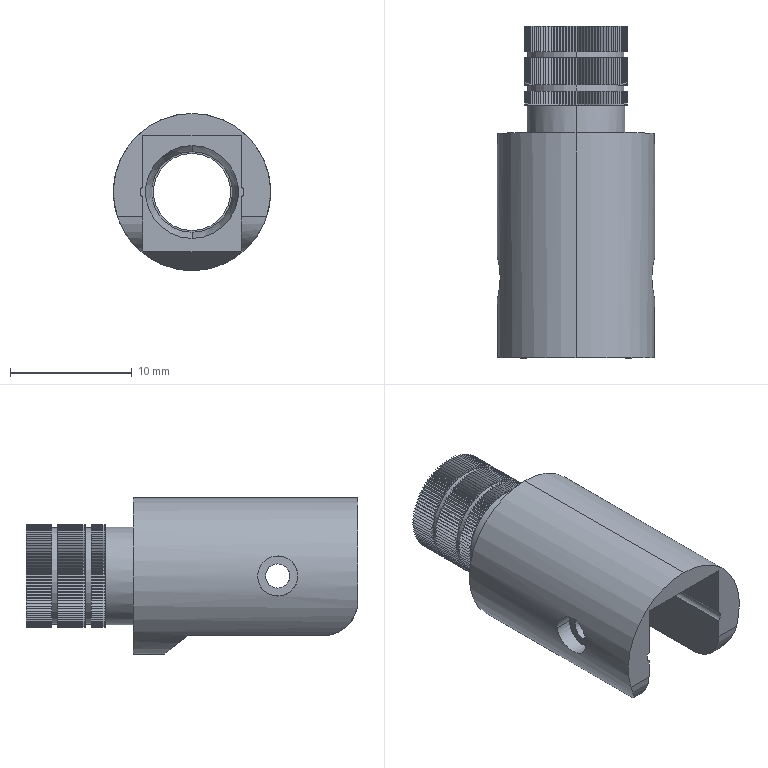Part | SolidWorks | features ICE 6, RevCut 2, Chamfer 1, Revolution 1 | 1 solid | 946 faces | box 12.92 x 27.3 x 12.92 mm | volume 1231 mm3 | plane 718 | cylinder 226 | cone 2 | commonest cylinder face diameters 8.06 x202 1 x4 2 x4 3.3 x4 7.96 x4 5.79 x2